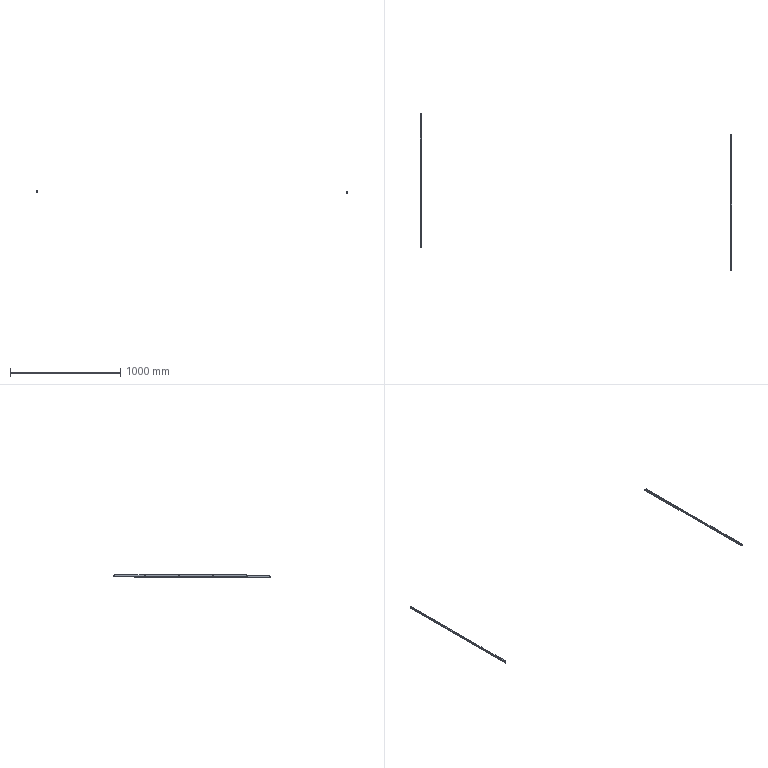NC program | NX | posted with a generic post | part box 2829 x 1430 x 20 mm
Whole program:
N10 G17 G21 G94 G90
(PLANAR_MILL_COPY , TOOL : D16-48-D16-100-3T-FINISH)
N12 T01 M6
N14 G54
N16 G17 G0 G90 X-526.5 Y0.5 S4000 M3
N18 G43 Z20. H1
N20 Z4.
N22 G94 G1 Z2. F1000.
N24 X-513.5
N26 X513.5
N28 X526.5
N30 Z4.
N32 G0 Z20.
N34 X-526.5
N36 Z3.
N38 G1 Z1.
N40 X-513.5
N42 X513.5
N44 X526.5
N46 Z3.
N48 G0 Z20.
N50 X-526.5
N52 Z2.1
N54 G1 Z0.1
N56 X-513.5
N58 X513.5
N60 X526.5
N62 Z2.1
N64 G0 Z20.
(PLANAR_MILL_COPY_COPY , TOOL : D16-48-D16-100-3T-FINISH)
N66 X-526.5
N68 Z2.
N70 G1 Z0.
N72 X-513.5
N74 X513.5
N76 X526.5
N78 Z2.
N80 G0 Z20.
N82 M5
(PLANAR_MILL_2 , TOOL : D8-25-D8-60-3T-FINISH)
N84 T03 M6
N86 G54
N88 G17 G0 G90 X-256.9 Y11. S4500 M3
N90 G43 Z20. H3
N92 Z1.5
N94 G94 G1 Z-0.5 F1200.
N96 Y5.
N98 Y-5.
N100 X-255.1
N102 Y5.
N104 Y11.
N106 Z1.5
N108 G0 X-256.9 Z1.
N110 G1 Z-1.
N112 Y5.
N114 Y-5.
N116 X-255.1
N118 Y5.
N120 Y11.
N122 Z1.
N124 G0 X-256.9 Z0.5
N126 G1 Z-1.5
N128 Y5.
N130 Y-5.
N132 X-255.1
N134 Y5.
N136 Y11.
N138 Z0.5
N140 G0 X-256.9 Z0.
N142 G1 Z-2.
N144 Y5.
N146 Y-5.
N148 X-255.1
N150 Y5.
N152 Y11.
N154 Z0.
N156 G0 X-256.9 Z-0.5
N158 G1 Z-2.5
N160 Y5.
N162 Y-5.
N164 X-255.1
N166 Y5.
N168 Y11.
N170 Z-0.5
N172 G0 X-256.9 Z-1.
N174 G1 Z-3.
N176 Y5.
N178 Y-5.
N180 X-255.1
N182 Y5.
N184 Y11.
N186 Z-1.
N188 G0 X-256.9 Z-1.5
N190 G1 Z-3.5
N192 Y5.
N194 Y-5.
N196 X-255.1
N198 Y5.
N200 Y11.
N202 Z-1.5
N204 G0 X-256.9 Z-2.
N206 G1 Z-4.
N208 Y5.
N210 Y-5.
N212 X-255.1
N214 Y5.
N216 Y11.
N218 Z-2.
N220 G0 X-256.9 Z-2.5
N222 G1 Z-4.5
N224 Y5.
N226 Y-5.
N228 X-255.1
N230 Y5.
N232 Y11.
N234 Z-2.5
N236 G0 X-256.9 Z-3.
N238 G1 Z-5.
N240 Y5.
N242 Y-5.
N244 X-255.1
N246 Y5.
N248 Y11.
N250 Z-3.
N252 G0 X-256.9 Z-3.5
N254 G1 Z-5.5
N256 Y5.
N258 Y-5.
N260 X-255.1
N262 Y5.
N264 Y11.
N266 Z-3.5
N268 G0 X-256.9 Z-4.
N270 G1 Z-6.
N272 Y5.
N274 Y-5.
N276 X-255.1
N278 Y5.
N280 Y11.
N282 Z-4.
N284 G0 X-256.9 Z-4.5
N286 G1 Z-6.5
N288 Y5.
N290 Y-5.
N292 X-255.1
N294 Y5.
N296 Y11.
N298 Z-4.5
N300 G0 X-256.9 Z-5.
N302 G1 Z-7.
N304 Y5.
N306 Y-5.
N308 X-255.1
N310 Y5.
N312 Y11.
N314 Z-5.
N316 G0 X-256.9 Z-5.5
N318 G1 Z-7.5
N320 Y5.
N322 Y-5.
N324 X-255.1
N326 Y5.
N328 Y11.
N330 Z-5.5
N332 G0 X-256.9 Z-5.9
N334 G1 Z-7.9
N336 Y5.
N338 Y-5.
N340 X-255.1
N342 Y5.
N344 Y11.
N346 Z-5.9
N348 G0 Z20.
N350 X-4.9
N352 Z1.5
N354 G1 Z-0.5
N356 Y5.
N358 Y-5.
N360 X-3.1
N362 Y5.
N364 Y11.
N366 Z1.5
N368 G0 X-4.9 Z1.
N370 G1 Z-1.
N372 Y5.
N374 Y-5.
N376 X-3.1
N378 Y5.
N380 Y11.
N382 Z1.
N384 G0 X-4.9 Z0.5
N386 G1 Z-1.5
N388 Y5.
N390 Y-5.
N392 X-3.1
N394 Y5.
N396 Y11.
N398 Z0.5
N400 G0 X-4.9 Z0.
N402 G1 Z-2.
N404 Y5.
N406 Y-5.
N408 X-3.1
N410 Y5.
N412 Y11.
N414 Z0.
N416 G0 X-4.9 Z-0.5
N418 G1 Z-2.5
N420 Y5.
N422 Y-5.
N424 X-3.1
N426 Y5.
N428 Y11.
N430 Z-0.5
N432 G0 X-4.9 Z-1.
N434 G1 Z-3.
N436 Y5.
N438 Y-5.
N440 X-3.1
N442 Y5.
N444 Y11.
N446 Z-1.
N448 G0 X-4.9 Z-1.5
N450 G1 Z-3.5
N452 Y5.
N454 Y-5.
N456 X-3.1
N458 Y5.
N460 Y11.
N462 Z-1.5
N464 G0 X-4.9 Z-2.
N466 G1 Z-4.
N468 Y5.
N470 Y-5.
N472 X-3.1
N474 Y5.
N476 Y11.
N478 Z-2.
N480 G0 X-4.9 Z-2.5
N482 G1 Z-4.5
N484 Y5.
N486 Y-5.
N488 X-3.1
N490 Y5.
N492 Y11.
N494 Z-2.5
N496 G0 X-4.9 Z-3.
N498 G1 Z-5.
N500 Y5.
N502 Y-5.
N504 X-3.1
N506 Y5.
N508 Y11.
N510 Z-3.
N512 G0 X-4.9 Z-3.5
N514 G1 Z-5.5
N516 Y5.
N518 Y-5.
N520 X-3.1
N522 Y5.
N524 Y11.
N526 Z-3.5
N528 G0 X-4.9 Z-4.
N530 G1 Z-6.
N532 Y5.
N534 Y-5.
N536 X-3.1
N538 Y5.
N540 Y11.
N542 Z-4.
N544 G0 X-4.9 Z-4.5
N546 G1 Z-6.5
N548 Y5.
N550 Y-5.
N552 X-3.1
N554 Y5.
N556 Y11.
N558 Z-4.5
N560 G0 X-4.9 Z-5.
N562 G1 Z-7.
N564 Y5.
N566 Y-5.
N568 X-3.1
N570 Y5.
N572 Y11.
N574 Z-5.
N576 G0 X-4.9 Z-5.5
N578 G1 Z-7.5
N580 Y5.
N582 Y-5.
N584 X-3.1
N586 Y5.
N588 Y11.
N590 Z-5.5
N592 G0 X-4.9 Z-5.9
N594 G1 Z-7.9
N596 Y5.
N598 Y-5.
N600 X-3.1
N602 Y5.
N604 Y11.
N606 Z-5.9
N608 G0 Z20.
N610 X255.1
N612 Z1.5
N614 G1 Z-0.5
N616 Y5.
N618 Y-5.
N620 X256.9
N622 Y5.
N624 Y11.
N626 Z1.5
N628 G0 X255.1 Z1.
N630 G1 Z-1.
N632 Y5.
N634 Y-5.
N636 X256.9
N638 Y5.
N640 Y11.
N642 Z1.
N644 G0 X255.1 Z0.5
N646 G1 Z-1.5
N648 Y5.
N650 Y-5.
N652 X256.9
N654 Y5.
N656 Y11.
N658 Z0.5
N660 G0 X255.1 Z0.
N662 G1 Z-2.
N664 Y5.
N666 Y-5.
N668 X256.9
N670 Y5.
N672 Y11.
N674 Z0.
N676 G0 X255.1 Z-0.5
N678 G1 Z-2.5
N680 Y5.
N682 Y-5.
N684 X256.9
N686 Y5.
N688 Y11.
N690 Z-0.5
N692 G0 X255.1 Z-1.
N694 G1 Z-3.
N696 Y5.
N698 Y-5.
N700 X256.9
N702 Y5.
N704 Y11.
N706 Z-1.
N708 G0 X255.1 Z-1.5
N710 G1 Z-3.5
N712 Y5.
N714 Y-5.
N716 X256.9
N718 Y5.
N720 Y11.
N722 Z-1.5
N724 G0 X255.1 Z-2.
N726 G1 Z-4.
N728 Y5.
N730 Y-5.
N732 X256.9
N734 Y5.
N736 Y11.
N738 Z-2.
N740 G0 X255.1 Z-2.5
N742 G1 Z-4.5
N744 Y5.
N746 Y-5.
N748 X256.9
N750 Y5.
N752 Y11.
N754 Z-2.5
N756 G0 X255.1 Z-3.
N758 G1 Z-5.
N760 Y5.
N762 Y-5.
N764 X256.9
N766 Y5.
N768 Y11.
N770 Z-3.
N772 G0 X255.1 Z-3.5
N774 G1 Z-5.5
N776 Y5.
N778 Y-5.
N780 X256.9
N782 Y5.
N784 Y11.
N786 Z-3.5
N788 G0 X255.1 Z-4.
N790 G1 Z-6.
N792 Y5.
N794 Y-5.
N796 X256.9
N798 Y5.
N800 Y11.
N802 Z-4.
N804 G0 X255.1 Z-4.5
N806 G1 Z-6.5
N808 Y5.
N810 Y-5.
N812 X256.9
N814 Y5.
N816 Y11.
N818 Z-4.5
N820 G0 X255.1 Z-5.
N822 G1 Z-7.
N824 Y5.
N826 Y-5.
N828 X256.9
N830 Y5.
N832 Y11.
N834 Z-5.
N836 G0 X255.1 Z-5.5
N838 G1 Z-7.5
N840 Y5.
N842 Y-5.
N844 X256.9
N846 Y5.
N848 Y11.
N850 Z-5.5
N852 G0 X255.1 Z-5.9
N854 G1 Z-7.9
N856 Y5.
N858 Y-5.
N860 X256.9
N862 Y5.
N864 Y11.
N866 Z-5.9
N868 G0 Z20.
(PLANAR_MILL_2_COPY , TOOL : D8-25-D8-60-3T-FINISH)
N870 X-256.846 Y11.985
N872 Z-6.
N874 G1 Z-8. F800.
N876 G41 X-257.02 Y11. D3
N878 Y5.
N880 Y-5.
N882 X-254.98
N884 Y5.
N886 Y11.
N888 G40
N890 X-255.154 Y11.985
N892 Z-6.
N894 G0 Z20.
N896 X-4.846
N898 Z-6.
N900 G1 Z-8.
N902 G41 X-5.02 Y11.
N904 Y5.
N906 Y-5.
N908 X-2.98
N910 Y5.
N912 Y11.
N914 G40
N916 X-3.154 Y11.985
N918 Z-6.
N920 G0 Z20.
N922 X255.154
N924 Z-6.
N926 G1 Z-8.
N928 G41 X254.98 Y11.
N930 Y5.
N932 Y-5.
N934 X257.02
N936 Y5.
N938 Y11.
N940 G40
N942 X256.846 Y11.985
N944 Z-6.
N946 G0 Z20.
N948 M5
(DRILLING , TOOL : 倒角D6-90度)
N950 T04 M6
N952 G54
N954 G17 G0 G90 X-498.75 Y0. S2000 M3
N956 G43 Z20. H4
N958 G94 G81 G99 Z-2. F200. R3.
N960 X-246.
N962 X6.
N964 X246.
N966 X498.75
N968 G80
N970 G0 X498.75 Y0. Z20.
(PLANAR_MILL_3 , TOOL : 倒角D6-90度)
N972 X384. Y8.5 S3000
N974 Z0.5
N976 G1 Z-1.5 F1000.
N978 G3 X386. Y6.5 R2.
N980 G1 X511.
N982 G2 X512.5 Y5. R1.5
N984 G1 Y-5.
N986 G2 X511. Y-6.5 R1.5
N988 G1 X261.
N990 G2 X259.5 Y-5. R1.5
N992 G1 Y5.
N994 G2 X261. Y6.5 R1.5
N996 G1 X386.
N998 G3 X388. Y8.5 R2.
N1000 G1 Z0.5
N1002 G0 Z20.
N1004 X124.
N1006 Z0.5
N1008 G1 Z-1.5
N1010 G3 X126. Y6.5 R2.
N1012 G1 X251.
N1014 G2 X252.5 Y5. R1.5
N1016 G1 Y-5.
N1018 G2 X251. Y-6.5 R1.5
N1020 G1 X1.
N1022 G2 X-0.5 Y-5. R1.5
N1024 G1 Y5.
N1026 G2 X1. Y6.5 R1.5
N1028 G1 X126.
N1030 G3 X128. Y8.5 R2.
N1032 G1 Z0.5
N1034 G0 Z20.
N1036 X-132.
N1038 Z0.5
N1040 G1 Z-1.5
N1042 G3 X-130. Y6.5 R2.
N1044 G1 X-9.
N1046 G2 X-7.5 Y5. R1.5
N1048 G1 Y-5.
N1050 G2 X-9. Y-6.5 R1.5
N1052 G1 X-251.
N1054 G2 X-252.5 Y-5. R1.5
N1056 G1 Y5.
N1058 G2 X-251. Y6.5 R1.5
N1060 G1 X-130.
N1062 G3 X-128. Y8.5 R2.
N1064 G1 Z0.5
N1066 G0 Z20.
N1068 X-388.
N1070 Z0.5
N1072 G1 Z-1.5
N1074 G3 X-386. Y6.5 R2.
N1076 G1 X-261.
N1078 G2 X-259.5 Y5. R1.5
N1080 G1 Y-5.
N1082 G2 X-261. Y-6.5 R1.5
N1084 G1 X-511.
N1086 G2 X-512.5 Y-5. R1.5
N1088 G1 Y5.
N1090 G2 X-511. Y6.5 R1.5
N1092 G1 X-386.
N1094 G3 X-384. Y8.5 R2.
N1096 G1 Z0.5
N1098 G0 Z20.
N1100 M5
(DRILLING_COPY , TOOL : 钻头D4.3-54-83)
N1102 T05 M6
N1104 G54
N1106 G17 G0 G90 X-498.75 Y0. S2000 M3
N1108 G43 Z20. H5
N1110 G94 G81 G98 Z-15. F200. R3.
N1112 X-246.
N1114 X6.
N1116 X246.
N1118 X498.75
N1120 G80
N1122 G0 X498.75 Y0. Z20.
N1124 M5
(DRILLING_COPY_COPY , TOOL : 上排M4-13-D5-52)
N1126 T06 M6
N1128 G54
N1130 G17 G0 G90 X-498.75 Y0. S300 M3
N1132 G43 Z20. H6
N1134 G84 G94 G98 Z-10. F210. R3.
N1136 X-246.
N1138 X6.
N1140 X246.
N1142 X498.75
N1144 G80
N1146 G0 X498.75 Y0. Z20.
N1148 M5
N1150 M2